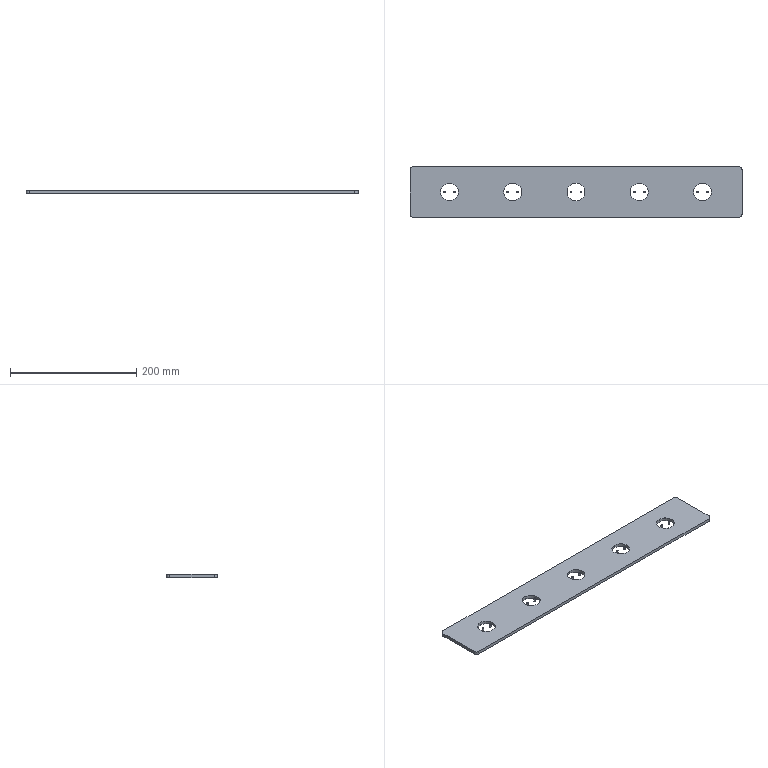Part | SolidWorks | features BaseBody 11 | 11 solids | 66 faces | box 525 x 80 x 5 mm | volume 194805 mm3 | cylinder 34 | plane 26 | torus 6 | commonest cylinder face diameters 2.794 x20 28 x10 10 x4